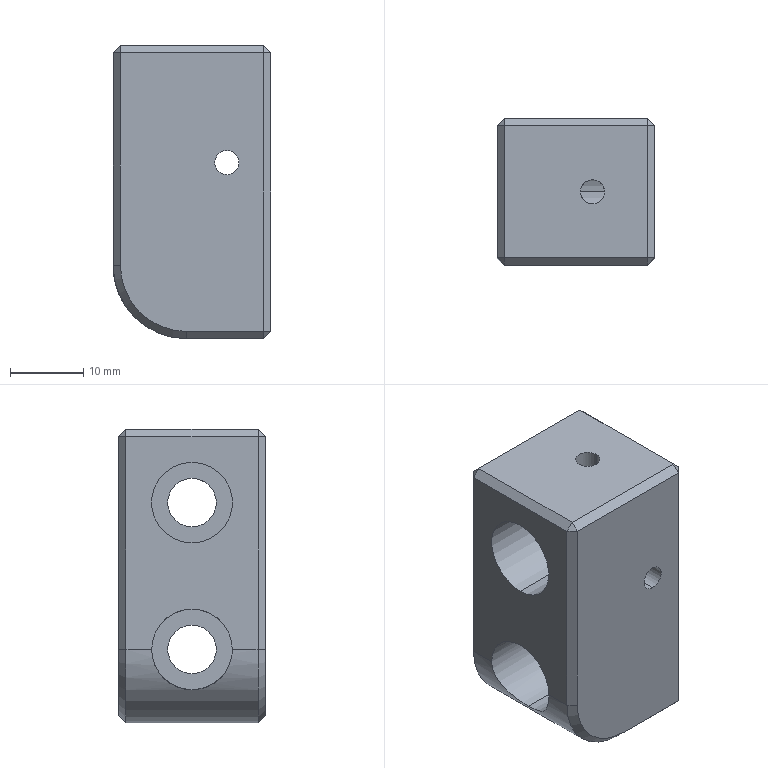Part | STEP file | 1 solid | 45 faces | box 21.5 x 20 x 40 mm | volume 13489 mm3 | plane 26 | cylinder 15 | cone 4 | commonest cylinder face diameters 3.3 x4 6.6 x4 11 x4 8.1 x2 20 x1